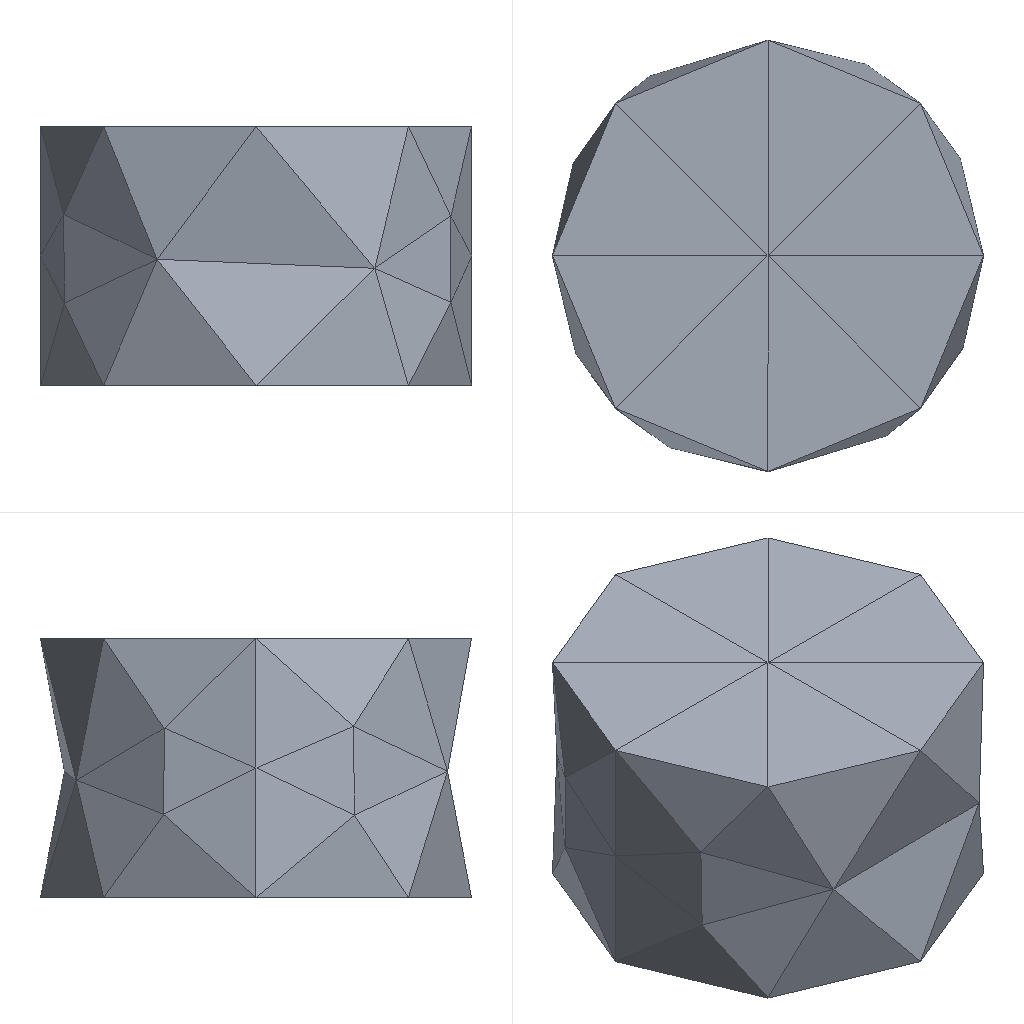Simulation study | ansys mapdl
Set-up summary:
category,name,step,type,value,unit,region
solver,ansys_mapdl
units,mm-N-s-tonne (MPa),,inferred,E=210000 density=
analysis,model,,static
mesh,nodes,,,198
mesh,elements,,,93
element_type,SOLID187,,,93
material,mat 1,,E,210000
material,mat 1,,nu,0.3
load,,model,body load temp,,,all
load,,model,force,"1000 [dir=(0, 0, -1) n=66]",,node list
bc,,model,fixed,"[dofs=UX,UY,UZ n=246]",,node list
Ansys APDL input file, long lists of numbers shortened:
/COM,ANSYS RELEASE 2026 R1           BUILD 26.1      UP20260202       09:11:09
/PREP7
/NOPR
/TITLE,2
ANTYPE, 0
*IF,_CDRDOFF,EQ,1,THEN     !if solid model was read in
_CDRDOFF=             !reset flag, numoffs already performed
*ELSE              !offset database for the following FE model
NUMOFF,NODE,      198
NUMOFF,ELEM,       93
NUMOFF,MAT ,        1
NUMOFF,TYPE,        1
*ENDIF
*SET,_RETURN ,  0.
*SET,_STATUS ,  0.
*SET,_UIQR   ,  66.
*SET,__FLOATPARAMETER__,  198.
DOF,DELETE
ETBLOCK,        1,        1
(2i9,19a9)
        1      187        0        0        0        0        0        0        0        0        0        0        0        0        0        0        0        0        0        0        0
       -1
NBLOCK,6,SOLID,       198,       198
(3i9,6e21.13e3)
        1        0        0-8.8817841970013E-016-1.0000000000000E+001 7.4000000000000E+001
! (197 more lines like these left out)
N,UNBL,LOC,       -1,
EBLOCK,19,SOLID,        93,        93
(19i10)
         1         1         1         1         0         0         0         0        10         0         1       123       121        52         6       129       104       130       131
! (185 more lines like these left out)
        -1
MPTEMP,UNBL, 1, 1,  0.    ,
MPDATA,UNBL, 1,EX  ,       1, 1,  210000.000    ,
MPTEMP,UNBL, 1, 1,  0.    ,
MPDATA,UNBL, 1,NUXY,       1, 1, 0.3    ,
MPTEMP,UNBL, 1, 1,  0.    ,
MPDATA,UNBL, 1,PRXY,       1, 1, 0.3    ,
EXTOPT,ATTR,      0,      0,      0
EXTOPT,ESIZE,  0,  0.
EXTOPT,ACLEAR,      0
TREF,  0.
IRLF,  0
BFUNIF,TEMP,_TINY
ACEL,  0.    ,  0.    ,  0.
OMEGA,  0.    ,  0.    ,  0.
DOMEGA,  0.    ,  0.    ,  0.
CGLOC,  0.    ,  0.    ,  0.
CGOMEGA,  0.    ,  0.    ,  0.
DCGOMG,  0.    ,  0.    ,  0.
KUSE,     0
TIME,  0.
ALPHAD,  0.
BETAD,  0.
DMPRAT,  0.
DMPSTR,  0.
CRPLIM, 0.1    ,   0
CRPLIM,  0.    ,   1
NCNV,     0, 1.000000000E+12,     0,  0.    ,  0.
NEQIT,     0
ERESX,DEFA
DBLOCK,       246
(i9,a6,2(pg16.9))
        1  UX    0.00000000      0.00000000
! (245 more lines like these left out)
       -1
FBLOCK,        66
(i9,a6,2(pg16.9))
       26  FZ   -15.1515152      0.00000000
! (65 more lines like these left out)
       -1
/GO
FINISH
Results summary:
result,analysis_type_db,,,static,unstated
result,n_sets,,,1,unstated
result,load_steps[0].set,load_step=1,,1,unstated
result,load_steps[0].substep,load_step=1,,1,unstated
result,load_steps[0].time,load_step=1,,1,unstated
result,load_steps[0].freq,load_step=1,,1,unstated
result,load_steps[0].max_usum,load_step=1,,0.000232,unstated
result,load_steps[0].max_seqv,load_step=1,,5.411,unstated
result,load_steps[0].reaction_sum.FX,load_step=1,,4.66827e-12,unstated
result,load_steps[0].reaction_sum.FY,load_step=1,,1.3074e-12,unstated
result,load_steps[0].reaction_sum.FZ,load_step=1,,1000,unstated
result,load_steps[0].reaction_sum.MX,load_step=1,,0,unstated
result,load_steps[0].reaction_sum.MY,load_step=1,,0,unstated
result,load_steps[0].reaction_sum.MZ,load_step=1,,0,unstated
result,convergence,,,results present for all listed sets,unstated